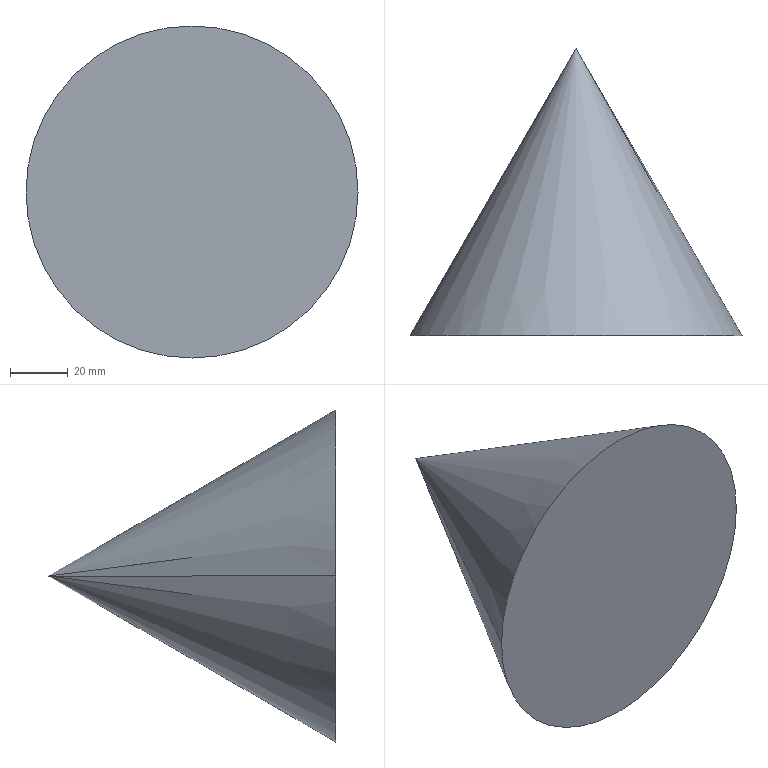Part | SolidWorks | features Revolution 1 | 1 solid | 3 faces | box 115.47 x 100 x 115.47 mm | volume 349066 mm3 | cone 2 | plane 1
STEP:
#1=CARTESIAN_POINT('',(0.,100.,0.));
#2=VERTEX_POINT('',#1);
#3=CARTESIAN_POINT('',(57.735,0.,0.));
#4=VERTEX_POINT('',#3);
#5=CARTESIAN_POINT('',(57.735,0.,0.));
#6=DIRECTION('',(0.5,-0.866,0.));
#7=VECTOR('',#6,1000.);
#8=LINE('',#5,#7);
#9=EDGE_CURVE('',#2,#4,#8,.T.);
#10=ORIENTED_EDGE('',*,*,#9,.F.);
#11=CARTESIAN_POINT('',(-57.735,0.,0.));
#12=VERTEX_POINT('',#11);
#13=CARTESIAN_POINT('',(-57.735,0.,0.));
#14=DIRECTION('',(-0.5,-0.866,0.));
#15=VECTOR('',#14,1000.);
#16=LINE('',#13,#15);
#17=EDGE_CURVE('',#2,#12,#16,.T.);
#18=ORIENTED_EDGE('',*,*,#17,.T.);
#19=CARTESIAN_POINT('',(0.,0.,0.));
#20=DIRECTION('',(0.,1.,0.));
#21=DIRECTION('',(-1.,0.,0.));
#22=AXIS2_PLACEMENT_3D('',#19,#20,#21);
#23=CIRCLE('',#22,57.735);
#24=EDGE_CURVE('',#12,#4,#23,.T.);
#25=ORIENTED_EDGE('',*,*,#24,.T.);
#26=EDGE_LOOP('',(#10,#18,#25));
#27=FACE_OUTER_BOUND('',#26,.T.);
#28=CARTESIAN_POINT('',(0.,0.,0.));
#29=DIRECTION('',(0.,-1.,0.));
#30=DIRECTION('',(1.,0.,0.));
#31=AXIS2_PLACEMENT_3D('',#28,#29,#30);
#32=CONICAL_SURFACE('',#31,57.735,0.5236);
#33=ADVANCED_FACE('',(#27),#32,.T.);
#34=CARTESIAN_POINT('',(0.,0.,0.));
#35=DIRECTION('',(0.,1.,0.));
#36=DIRECTION('',(-1.,0.,0.));
#37=AXIS2_PLACEMENT_3D('',#34,#35,#36);
#38=CIRCLE('',#37,57.735);
#39=EDGE_CURVE('',#4,#12,#38,.T.);
#40=ORIENTED_EDGE('',*,*,#39,.F.);
#41=ORIENTED_EDGE('',*,*,#24,.F.);
#42=EDGE_LOOP('',(#40,#41));
#43=FACE_OUTER_BOUND('',#42,.T.);
#44=CARTESIAN_POINT('',(0.,0.,0.));
#45=DIRECTION('',(0.,1.,0.));
#46=DIRECTION('',(-1.,0.,0.));
#47=AXIS2_PLACEMENT_3D('',#44,#45,#46);
#48=PLANE('',#47);
#49=ADVANCED_FACE('',(#43),#48,.F.);
#50=ORIENTED_EDGE('',*,*,#17,.F.);
#51=ORIENTED_EDGE('',*,*,#9,.T.);
#52=ORIENTED_EDGE('',*,*,#39,.T.);
#53=EDGE_LOOP('',(#50,#51,#52));
#54=FACE_OUTER_BOUND('',#53,.T.);
#55=CARTESIAN_POINT('',(0.,0.,0.));
#56=DIRECTION('',(0.,-1.,0.));
#57=DIRECTION('',(1.,0.,0.));
#58=AXIS2_PLACEMENT_3D('',#55,#56,#57);
#59=CONICAL_SURFACE('',#58,57.735,0.5236);
#60=ADVANCED_FACE('',(#54),#59,.T.);
#61=CLOSED_SHELL('',(#33,#49,#60));
#62=MANIFOLD_SOLID_BREP('',#61);
#63=CARTESIAN_POINT('',(0.,0.,0.));
#64=DIRECTION('',(0.,0.,1.));
#65=DIRECTION('',(1.,0.,0.));
#66=AXIS2_PLACEMENT_3D('',#63,#64,#65);
#67=(LENGTH_UNIT()NAMED_UNIT(*)SI_UNIT(.MILLI.,.METRE.));
#68=UNCERTAINTY_MEASURE_WITH_UNIT(LENGTH_MEASURE(0.00001),#67,'','');
#69=(NAMED_UNIT(*)PLANE_ANGLE_UNIT()SI_UNIT($,.RADIAN.));
#70=(NAMED_UNIT(*)SI_UNIT($,.STERADIAN.)SOLID_ANGLE_UNIT());
#71=(GEOMETRIC_REPRESENTATION_CONTEXT(3)GLOBAL_UNCERTAINTY_ASSIGNED_CONTEXT((#68))GLOBAL_UNIT_ASSIGNED_CONTEXT((#67,#69,#70))REPRESENTATION_CONTEXT('',''));
#72=ADVANCED_BREP_SHAPE_REPRESENTATION('',(#62,#66),#71);